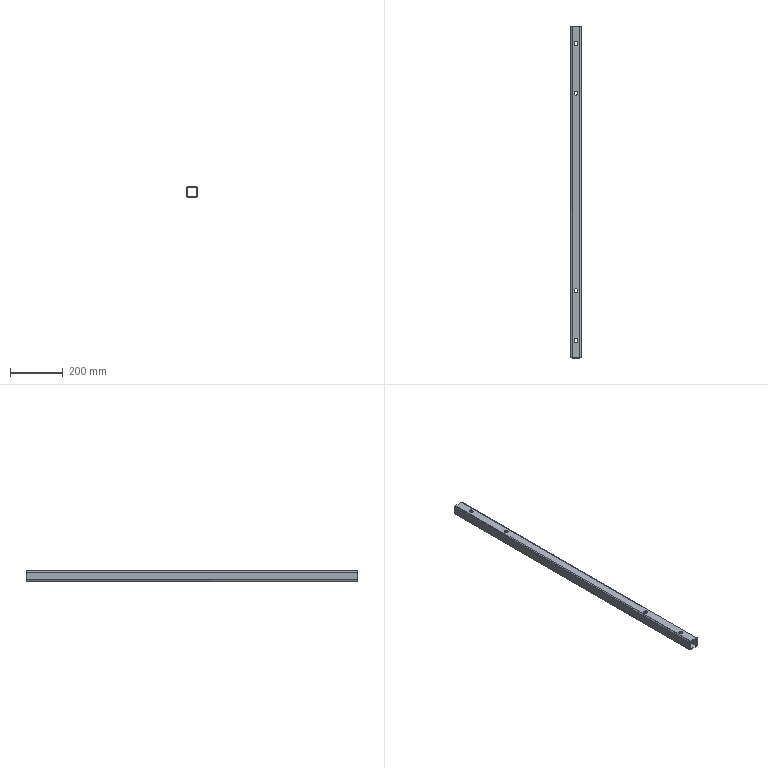Part | NX | features BREP 1 | 1 solid | 52 faces | box 40 x 1258 x 40 mm | volume 362402 mm3 | cylinder 28 | plane 24 | commonest cylinder face diameters 15 x16 6 x8 10 x4